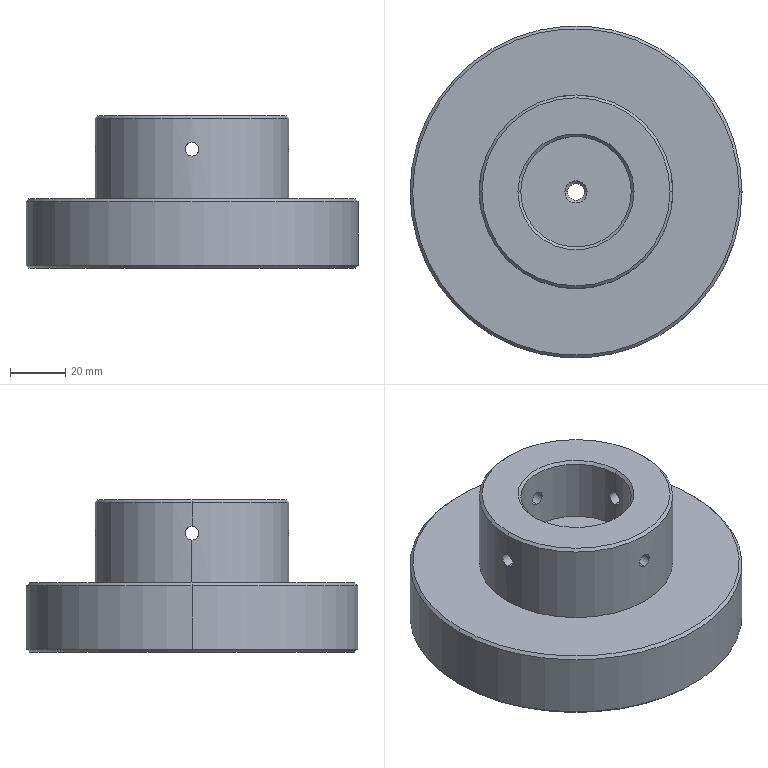Part | STEP file | 001-009-Riveting mechanism upper die holder | 1 solid | 37 faces | box 120 x 120 x 55 mm | volume 359662 mm3 | cylinder 18 | cone 14 | plane 5 | commonest cylinder face diameters 5 x8 6 x2 20 x2 40 x2 70 x2 120 x2